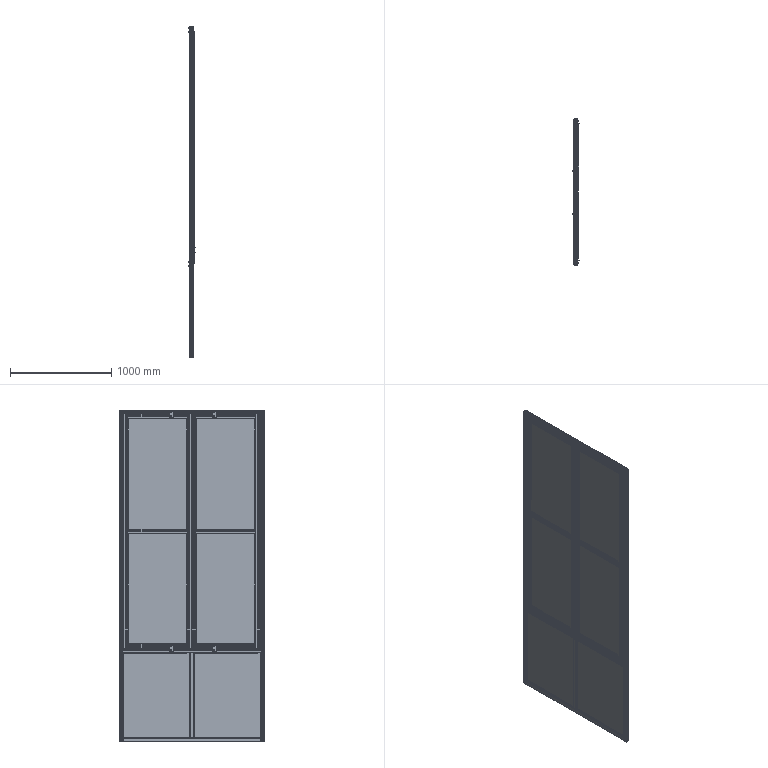Part | SolidWorks | 237 solids | 13281 faces | volume 36484784 mm3 | plane 6358 | cylinder 6258 | cone 619 | spline 46 | commonest cylinder face diameters 4 x3696 0.6 x320 10 x240 6.6 x232 8 x192 6.8 x185